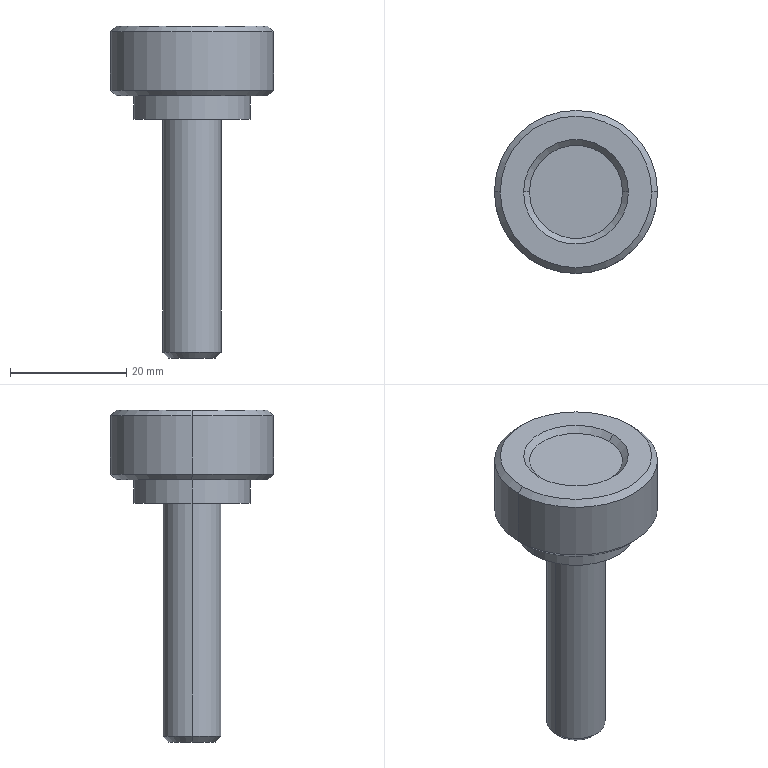Part | STEP file | Screen clamp adjusting handle | 1 solid | 23 faces | box 28 x 28 x 57 mm | volume 11437 mm3 | cone 10 | cylinder 8 | plane 5 | commonest cylinder face diameters 3.3 x2 10 x2 20 x2 28 x2
STEP:
#1=CARTESIAN_POINT('',(1.65,0.,-33.5));
#2=VERTEX_POINT('',#1);
#3=CARTESIAN_POINT('',(-1.65,0.,-33.5));
#4=VERTEX_POINT('',#3);
#5=CARTESIAN_POINT('',(0.,0.,-33.5));
#6=DIRECTION('',(0.,0.,-1.));
#7=DIRECTION('',(-1.,0.,0.));
#8=AXIS2_PLACEMENT_3D('',#5,#6,#7);
#9=CIRCLE('',#8,1.65);
#10=EDGE_CURVE('',#2,#4,#9,.T.);
#11=ORIENTED_EDGE('',*,*,#10,.F.);
#12=CARTESIAN_POINT('',(1.65,0.,-45.));
#13=VERTEX_POINT('',#12);
#14=CARTESIAN_POINT('',(1.65,0.,-45.));
#15=DIRECTION('',(0.,0.,-1.));
#16=VECTOR('',#15,1000.);
#17=LINE('',#14,#16);
#18=EDGE_CURVE('',#2,#13,#17,.T.);
#19=ORIENTED_EDGE('',*,*,#18,.T.);
#20=CARTESIAN_POINT('',(-1.65,0.,-45.));
#21=VERTEX_POINT('',#20);
#22=CARTESIAN_POINT('',(0.,0.,-45.));
#23=DIRECTION('',(0.,0.,-1.));
#24=DIRECTION('',(-1.,0.,0.));
#25=AXIS2_PLACEMENT_3D('',#22,#23,#24);
#26=CIRCLE('',#25,1.65);
#27=EDGE_CURVE('',#13,#21,#26,.T.);
#28=ORIENTED_EDGE('',*,*,#27,.T.);
#29=CARTESIAN_POINT('',(-1.65,0.,-45.));
#30=DIRECTION('',(0.,0.,-1.));
#31=VECTOR('',#30,1000.);
#32=LINE('',#29,#31);
#33=EDGE_CURVE('',#4,#21,#32,.T.);
#34=ORIENTED_EDGE('',*,*,#33,.F.);
#35=EDGE_LOOP('',(#11,#19,#28,#34));
#36=FACE_OUTER_BOUND('',#35,.T.);
#37=CARTESIAN_POINT('',(0.,0.,-45.));
#38=DIRECTION('',(0.,0.,-1.));
#39=DIRECTION('',(-1.,0.,0.));
#40=AXIS2_PLACEMENT_3D('',#37,#38,#39);
#41=CYLINDRICAL_SURFACE('',#40,1.65);
#42=ADVANCED_FACE('',(#36),#41,.F.);
#43=CARTESIAN_POINT('',(0.,0.,-32.509));
#44=VERTEX_POINT('',#43);
#45=CARTESIAN_POINT('',(-1.65,0.,-33.5));
#46=DIRECTION('',(-0.8572,0.,-0.515));
#47=VECTOR('',#46,1000.);
#48=LINE('',#45,#47);
#49=EDGE_CURVE('',#44,#4,#48,.T.);
#50=ORIENTED_EDGE('',*,*,#49,.F.);
#51=CARTESIAN_POINT('',(1.65,0.,-33.5));
#52=DIRECTION('',(0.8572,0.,-0.515));
#53=VECTOR('',#52,1000.);
#54=LINE('',#51,#53);
#55=EDGE_CURVE('',#44,#2,#54,.T.);
#56=ORIENTED_EDGE('',*,*,#55,.T.);
#57=ORIENTED_EDGE('',*,*,#10,.T.);
#58=EDGE_LOOP('',(#50,#56,#57));
#59=FACE_OUTER_BOUND('',#58,.T.);
#60=CARTESIAN_POINT('',(0.,0.,-33.5));
#61=DIRECTION('',(0.,0.,-1.));
#62=DIRECTION('',(-1.,0.,0.));
#63=AXIS2_PLACEMENT_3D('',#60,#61,#62);
#64=CONICAL_SURFACE('',#63,1.65,1.03);
#65=ADVANCED_FACE('',(#59),#64,.F.);
#66=CARTESIAN_POINT('',(-4.,0.,-45.));
#67=VERTEX_POINT('',#66);
#68=CARTESIAN_POINT('',(4.,0.,-45.));
#69=VERTEX_POINT('',#68);
#70=CARTESIAN_POINT('',(0.,0.,-45.));
#71=DIRECTION('',(0.,0.,-1.));
#72=DIRECTION('',(-1.,0.,0.));
#73=AXIS2_PLACEMENT_3D('',#70,#71,#72);
#74=CIRCLE('',#73,4.);
#75=EDGE_CURVE('',#67,#69,#74,.T.);
#76=ORIENTED_EDGE('',*,*,#75,.F.);
#77=CARTESIAN_POINT('',(-5.,0.,-44.));
#78=VERTEX_POINT('',#77);
#79=CARTESIAN_POINT('',(-4.,0.,-45.));
#80=DIRECTION('',(-0.7071,0.,0.7071));
#81=VECTOR('',#80,1000.);
#82=LINE('',#79,#81);
#83=EDGE_CURVE('',#67,#78,#82,.T.);
#84=ORIENTED_EDGE('',*,*,#83,.T.);
#85=CARTESIAN_POINT('',(5.,0.,-44.));
#86=VERTEX_POINT('',#85);
#87=CARTESIAN_POINT('',(0.,0.,-44.));
#88=DIRECTION('',(0.,0.,1.));
#89=DIRECTION('',(-1.,0.,0.));
#90=AXIS2_PLACEMENT_3D('',#87,#88,#89);
#91=CIRCLE('',#90,5.);
#92=EDGE_CURVE('',#86,#78,#91,.T.);
#93=ORIENTED_EDGE('',*,*,#92,.F.);
#94=CARTESIAN_POINT('',(4.,0.,-45.));
#95=DIRECTION('',(0.7071,0.,0.7071));
#96=VECTOR('',#95,1000.);
#97=LINE('',#94,#96);
#98=EDGE_CURVE('',#69,#86,#97,.T.);
#99=ORIENTED_EDGE('',*,*,#98,.F.);
#100=EDGE_LOOP('',(#76,#84,#93,#99));
#101=FACE_OUTER_BOUND('',#100,.T.);
#102=CARTESIAN_POINT('',(0.,0.,-45.));
#103=DIRECTION('',(0.,0.,1.));
#104=DIRECTION('',(1.,0.,0.));
#105=AXIS2_PLACEMENT_3D('',#102,#103,#104);
#106=CONICAL_SURFACE('',#105,4.,0.7854);
#107=ADVANCED_FACE('',(#101),#106,.T.);
#108=CARTESIAN_POINT('',(-13.,0.,0.));
#109=VERTEX_POINT('',#108);
#110=CARTESIAN_POINT('',(13.,0.,0.));
#111=VERTEX_POINT('',#110);
#112=CARTESIAN_POINT('',(0.,0.,0.));
#113=DIRECTION('',(0.,0.,-1.));
#114=DIRECTION('',(1.,0.,0.));
#115=AXIS2_PLACEMENT_3D('',#112,#113,#114);
#116=CIRCLE('',#115,13.);
#117=EDGE_CURVE('',#109,#111,#116,.T.);
#118=ORIENTED_EDGE('',*,*,#117,.F.);
#119=CARTESIAN_POINT('',(-14.,0.,1.));
#120=VERTEX_POINT('',#119);
#121=CARTESIAN_POINT('',(-14.,0.,1.));
#122=DIRECTION('',(-0.7071,0.,0.7071));
#123=VECTOR('',#122,1000.);
#124=LINE('',#121,#123);
#125=EDGE_CURVE('',#109,#120,#124,.T.);
#126=ORIENTED_EDGE('',*,*,#125,.T.);
#127=CARTESIAN_POINT('',(14.,0.,1.));
#128=VERTEX_POINT('',#127);
#129=CARTESIAN_POINT('',(0.,0.,1.));
#130=DIRECTION('',(0.,0.,1.));
#131=DIRECTION('',(1.,0.,0.));
#132=AXIS2_PLACEMENT_3D('',#129,#130,#131);
#133=CIRCLE('',#132,14.);
#134=EDGE_CURVE('',#128,#120,#133,.T.);
#135=ORIENTED_EDGE('',*,*,#134,.F.);
#136=CARTESIAN_POINT('',(14.,0.,1.));
#137=DIRECTION('',(0.7071,0.,0.7071));
#138=VECTOR('',#137,1000.);
#139=LINE('',#136,#138);
#140=EDGE_CURVE('',#111,#128,#139,.T.);
#141=ORIENTED_EDGE('',*,*,#140,.F.);
#142=EDGE_LOOP('',(#118,#126,#135,#141));
#143=FACE_OUTER_BOUND('',#142,.T.);
#144=CARTESIAN_POINT('',(0.,0.,1.));
#145=DIRECTION('',(0.,0.,1.));
#146=DIRECTION('',(1.,0.,0.));
#147=AXIS2_PLACEMENT_3D('',#144,#145,#146);
#148=CONICAL_SURFACE('',#147,14.,0.7854);
#149=ADVANCED_FACE('',(#143),#148,.T.);
#150=CARTESIAN_POINT('',(13.,0.,12.));
#151=VERTEX_POINT('',#150);
#152=CARTESIAN_POINT('',(-13.,0.,12.));
#153=VERTEX_POINT('',#152);
#154=CARTESIAN_POINT('',(0.,0.,12.));
#155=DIRECTION('',(0.,0.,1.));
#156=DIRECTION('',(1.,0.,0.));
#157=AXIS2_PLACEMENT_3D('',#154,#155,#156);
#158=CIRCLE('',#157,13.);
#159=EDGE_CURVE('',#151,#153,#158,.T.);
#160=ORIENTED_EDGE('',*,*,#159,.F.);
#161=CARTESIAN_POINT('',(14.,0.,11.));
#162=VERTEX_POINT('',#161);
#163=CARTESIAN_POINT('',(13.,0.,12.));
#164=DIRECTION('',(0.7071,0.,-0.7071));
#165=VECTOR('',#164,1000.);
#166=LINE('',#163,#165);
#167=EDGE_CURVE('',#151,#162,#166,.T.);
#168=ORIENTED_EDGE('',*,*,#167,.T.);
#169=CARTESIAN_POINT('',(-14.,0.,11.));
#170=VERTEX_POINT('',#169);
#171=CARTESIAN_POINT('',(0.,0.,11.));
#172=DIRECTION('',(0.,0.,-1.));
#173=DIRECTION('',(1.,0.,0.));
#174=AXIS2_PLACEMENT_3D('',#171,#172,#173);
#175=CIRCLE('',#174,14.);
#176=EDGE_CURVE('',#170,#162,#175,.T.);
#177=ORIENTED_EDGE('',*,*,#176,.F.);
#178=CARTESIAN_POINT('',(-13.,0.,12.));
#179=DIRECTION('',(-0.7071,0.,-0.7071));
#180=VECTOR('',#179,1000.);
#181=LINE('',#178,#180);
#182=EDGE_CURVE('',#153,#170,#181,.T.);
#183=ORIENTED_EDGE('',*,*,#182,.F.);
#184=EDGE_LOOP('',(#160,#168,#177,#183));
#185=FACE_OUTER_BOUND('',#184,.T.);
#186=CARTESIAN_POINT('',(0.,0.,12.));
#187=DIRECTION('',(0.,0.,-1.));
#188=DIRECTION('',(-1.,0.,0.));
#189=AXIS2_PLACEMENT_3D('',#186,#187,#188);
#190=CONICAL_SURFACE('',#189,13.,0.7854);
#191=ADVANCED_FACE('',(#185),#190,.T.);
#192=CARTESIAN_POINT('',(-8.,0.,11.));
#193=VERTEX_POINT('',#192);
#194=CARTESIAN_POINT('',(8.,0.,11.));
#195=VERTEX_POINT('',#194);
#196=CARTESIAN_POINT('',(0.,0.,11.));
#197=DIRECTION('',(0.,0.,1.));
#198=DIRECTION('',(1.,0.,0.));
#199=AXIS2_PLACEMENT_3D('',#196,#197,#198);
#200=CIRCLE('',#199,8.);
#201=EDGE_CURVE('',#193,#195,#200,.T.);
#202=ORIENTED_EDGE('',*,*,#201,.F.);
#203=CARTESIAN_POINT('',(-9.,0.,12.));
#204=VERTEX_POINT('',#203);
#205=CARTESIAN_POINT('',(-8.,0.,11.));
#206=DIRECTION('',(-0.7071,0.,0.7071));
#207=VECTOR('',#206,1000.);
#208=LINE('',#205,#207);
#209=EDGE_CURVE('',#193,#204,#208,.T.);
#210=ORIENTED_EDGE('',*,*,#209,.T.);
#211=CARTESIAN_POINT('',(9.,0.,12.));
#212=VERTEX_POINT('',#211);
#213=CARTESIAN_POINT('',(0.,0.,12.));
#214=DIRECTION('',(0.,0.,-1.));
#215=DIRECTION('',(1.,0.,0.));
#216=AXIS2_PLACEMENT_3D('',#213,#214,#215);
#217=CIRCLE('',#216,9.);
#218=EDGE_CURVE('',#212,#204,#217,.T.);
#219=ORIENTED_EDGE('',*,*,#218,.F.);
#220=CARTESIAN_POINT('',(8.,0.,11.));
#221=DIRECTION('',(0.7071,0.,0.7071));
#222=VECTOR('',#221,1000.);
#223=LINE('',#220,#222);
#224=EDGE_CURVE('',#195,#212,#223,.T.);
#225=ORIENTED_EDGE('',*,*,#224,.F.);
#226=EDGE_LOOP('',(#202,#210,#219,#225));
#227=FACE_OUTER_BOUND('',#226,.T.);
#228=CARTESIAN_POINT('',(0.,0.,11.));
#229=DIRECTION('',(0.,0.,1.));
#230=DIRECTION('',(1.,0.,0.));
#231=AXIS2_PLACEMENT_3D('',#228,#229,#230);
#232=CONICAL_SURFACE('',#231,8.,0.7854);
#233=ADVANCED_FACE('',(#227),#232,.F.);
#234=ORIENTED_EDGE('',*,*,#92,.T.);
#235=CARTESIAN_POINT('',(-5.,0.,-4.));
#236=VERTEX_POINT('',#235);
#237=CARTESIAN_POINT('',(-5.,0.,-45.));
#238=DIRECTION('',(0.,0.,1.));
#239=VECTOR('',#238,1000.);
#240=LINE('',#237,#239);
#241=EDGE_CURVE('',#78,#236,#240,.T.);
#242=ORIENTED_EDGE('',*,*,#241,.T.);
#243=CARTESIAN_POINT('',(5.,0.,-4.));
#244=VERTEX_POINT('',#243);
#245=CARTESIAN_POINT('',(0.,0.,-4.));
#246=DIRECTION('',(0.,0.,-1.));
#247=DIRECTION('',(-1.,0.,0.));
#248=AXIS2_PLACEMENT_3D('',#245,#246,#247);
#249=CIRCLE('',#248,5.);
#250=EDGE_CURVE('',#236,#244,#249,.T.);
#251=ORIENTED_EDGE('',*,*,#250,.T.);
#252=CARTESIAN_POINT('',(5.,0.,-45.));
#253=DIRECTION('',(0.,0.,1.));
#254=VECTOR('',#253,1000.);
#255=LINE('',#252,#254);
#256=EDGE_CURVE('',#86,#244,#255,.T.);
#257=ORIENTED_EDGE('',*,*,#256,.F.);
#258=EDGE_LOOP('',(#234,#242,#251,#257));
#259=FACE_OUTER_BOUND('',#258,.T.);
#260=CARTESIAN_POINT('',(0.,0.,-45.));
#261=DIRECTION('',(0.,0.,1.));
#262=DIRECTION('',(1.,0.,0.));
#263=AXIS2_PLACEMENT_3D('',#260,#261,#262);
#264=CYLINDRICAL_SURFACE('',#263,5.);
#265=ADVANCED_FACE('',(#259),#264,.T.);
#266=CARTESIAN_POINT('',(-10.,0.,-4.));
#267=VERTEX_POINT('',#266);
#268=CARTESIAN_POINT('',(10.,0.,-4.));
#269=VERTEX_POINT('',#268);
#270=CARTESIAN_POINT('',(0.,0.,-4.));
#271=DIRECTION('',(0.,0.,-1.));
#272=DIRECTION('',(-1.,0.,0.));
#273=AXIS2_PLACEMENT_3D('',#270,#271,#272);
#274=CIRCLE('',#273,10.);
#275=EDGE_CURVE('',#267,#269,#274,.T.);
#276=ORIENTED_EDGE('',*,*,#275,.F.);
#277=CARTESIAN_POINT('',(-10.,0.,0.));
#278=VERTEX_POINT('',#277);
#279=CARTESIAN_POINT('',(-10.,0.,-4.));
#280=DIRECTION('',(0.,0.,1.));
#281=VECTOR('',#280,1000.);
#282=LINE('',#279,#281);
#283=EDGE_CURVE('',#267,#278,#282,.T.);
#284=ORIENTED_EDGE('',*,*,#283,.T.);
#285=CARTESIAN_POINT('',(10.,0.,0.));
#286=VERTEX_POINT('',#285);
#287=CARTESIAN_POINT('',(0.,0.,0.));
#288=DIRECTION('',(0.,0.,-1.));
#289=DIRECTION('',(1.,0.,0.));
#290=AXIS2_PLACEMENT_3D('',#287,#288,#289);
#291=CIRCLE('',#290,10.);
#292=EDGE_CURVE('',#278,#286,#291,.T.);
#293=ORIENTED_EDGE('',*,*,#292,.T.);
#294=CARTESIAN_POINT('',(10.,0.,-4.));
#295=DIRECTION('',(0.,0.,1.));
#296=VECTOR('',#295,1000.);
#297=LINE('',#294,#296);
#298=EDGE_CURVE('',#269,#286,#297,.T.);
#299=ORIENTED_EDGE('',*,*,#298,.F.);
#300=EDGE_LOOP('',(#276,#284,#293,#299));
#301=FACE_OUTER_BOUND('',#300,.T.);
#302=CARTESIAN_POINT('',(0.,0.,-4.));
#303=DIRECTION('',(0.,0.,1.));
#304=DIRECTION('',(1.,0.,0.));
#305=AXIS2_PLACEMENT_3D('',#302,#303,#304);
#306=CYLINDRICAL_SURFACE('',#305,10.);
#307=ADVANCED_FACE('',(#301),#306,.T.);
#308=ORIENTED_EDGE('',*,*,#176,.T.);
#309=CARTESIAN_POINT('',(14.,0.,12.));
#310=DIRECTION('',(0.,0.,-1.));
#311=VECTOR('',#310,1000.);
#312=LINE('',#309,#311);
#313=EDGE_CURVE('',#162,#128,#312,.T.);
#314=ORIENTED_EDGE('',*,*,#313,.T.);
#315=ORIENTED_EDGE('',*,*,#134,.T.);
#316=CARTESIAN_POINT('',(-14.,0.,12.));
#317=DIRECTION('',(0.,0.,-1.));
#318=VECTOR('',#317,1000.);
#319=LINE('',#316,#318);
#320=EDGE_CURVE('',#170,#120,#319,.T.);
#321=ORIENTED_EDGE('',*,*,#320,.F.);
#322=EDGE_LOOP('',(#308,#314,#315,#321));
#323=FACE_OUTER_BOUND('',#322,.T.);
#324=CARTESIAN_POINT('',(0.,0.,12.));
#325=DIRECTION('',(0.,0.,-1.));
#326=DIRECTION('',(-1.,0.,0.));
#327=AXIS2_PLACEMENT_3D('',#324,#325,#326);
#328=CYLINDRICAL_SURFACE('',#327,14.);
#329=ADVANCED_FACE('',(#323),#328,.T.);
#330=CARTESIAN_POINT('',(0.,0.,0.));
#331=DIRECTION('',(0.,0.,-1.));
#332=DIRECTION('',(1.,0.,0.));
#333=AXIS2_PLACEMENT_3D('',#330,#331,#332);
#334=CIRCLE('',#333,13.);
#335=EDGE_CURVE('',#111,#109,#334,.T.);
#336=ORIENTED_EDGE('',*,*,#335,.T.);
#337=ORIENTED_EDGE('',*,*,#117,.T.);
#338=EDGE_LOOP('',(#336,#337));
#339=FACE_OUTER_BOUND('',#338,.T.);
#340=CARTESIAN_POINT('',(0.,0.,0.));
#341=DIRECTION('',(0.,0.,-1.));
#342=DIRECTION('',(1.,0.,0.));
#343=AXIS2_PLACEMENT_3D('',#340,#341,#342);
#344=CIRCLE('',#343,10.);
#345=EDGE_CURVE('',#286,#278,#344,.T.);
#346=ORIENTED_EDGE('',*,*,#345,.F.);
#347=ORIENTED_EDGE('',*,*,#292,.F.);
#348=EDGE_LOOP('',(#346,#347));
#349=FACE_BOUND('',#348,.T.);
#350=CARTESIAN_POINT('',(0.,0.,0.));
#351=DIRECTION('',(0.,0.,1.));
#352=DIRECTION('',(1.,0.,0.));
#353=AXIS2_PLACEMENT_3D('',#350,#351,#352);
#354=PLANE('',#353);
#355=ADVANCED_FACE('',(#339,#349),#354,.F.);
#356=ORIENTED_EDGE('',*,*,#313,.F.);
#357=CARTESIAN_POINT('',(0.,0.,11.));
#358=DIRECTION('',(0.,0.,-1.));
#359=DIRECTION('',(1.,0.,0.));
#360=AXIS2_PLACEMENT_3D('',#357,#358,#359);
#361=CIRCLE('',#360,14.);
#362=EDGE_CURVE('',#162,#170,#361,.T.);
#363=ORIENTED_EDGE('',*,*,#362,.T.);
#364=ORIENTED_EDGE('',*,*,#320,.T.);
#365=CARTESIAN_POINT('',(0.,0.,1.));
#366=DIRECTION('',(0.,0.,1.));
#367=DIRECTION('',(1.,0.,0.));
#368=AXIS2_PLACEMENT_3D('',#365,#366,#367);
#369=CIRCLE('',#368,14.);
#370=EDGE_CURVE('',#120,#128,#369,.T.);
#371=ORIENTED_EDGE('',*,*,#370,.T.);
#372=EDGE_LOOP('',(#356,#363,#364,#371));
#373=FACE_OUTER_BOUND('',#372,.T.);
#374=CARTESIAN_POINT('',(0.,0.,12.));
#375=DIRECTION('',(0.,0.,-1.));
#376=DIRECTION('',(-1.,0.,0.));
#377=AXIS2_PLACEMENT_3D('',#374,#375,#376);
#378=CYLINDRICAL_SURFACE('',#377,14.);
#379=ADVANCED_FACE('',(#373),#378,.T.);
#380=ORIENTED_EDGE('',*,*,#218,.T.);
#381=CARTESIAN_POINT('',(0.,0.,12.));
#382=DIRECTION('',(0.,0.,-1.));
#383=DIRECTION('',(1.,0.,0.));
#384=AXIS2_PLACEMENT_3D('',#381,#382,#383);
#385=CIRCLE('',#384,9.);
#386=EDGE_CURVE('',#204,#212,#385,.T.);
#387=ORIENTED_EDGE('',*,*,#386,.T.);
#388=EDGE_LOOP('',(#380,#387));
#389=FACE_BOUND('',#388,.T.);
#390=CARTESIAN_POINT('',(0.,0.,12.));
#391=DIRECTION('',(0.,0.,1.));
#392=DIRECTION('',(1.,0.,0.));
#393=AXIS2_PLACEMENT_3D('',#390,#391,#392);
#394=CIRCLE('',#393,13.);
#395=EDGE_CURVE('',#153,#151,#394,.T.);
#396=ORIENTED_EDGE('',*,*,#395,.T.);
#397=ORIENTED_EDGE('',*,*,#159,.T.);
#398=EDGE_LOOP('',(#396,#397));
#399=FACE_OUTER_BOUND('',#398,.T.);
#400=CARTESIAN_POINT('',(0.,0.,12.));
#401=DIRECTION('',(0.,0.,1.));
#402=DIRECTION('',(1.,0.,0.));
#403=AXIS2_PLACEMENT_3D('',#400,#401,#402);
#404=PLANE('',#403);
#405=ADVANCED_FACE('',(#389,#399),#404,.T.);
#406=CARTESIAN_POINT('',(0.,0.,-4.));
#407=DIRECTION('',(0.,0.,-1.));
#408=DIRECTION('',(-1.,0.,0.));
#409=AXIS2_PLACEMENT_3D('',#406,#407,#408);
#410=CIRCLE('',#409,10.);
#411=EDGE_CURVE('',#269,#267,#410,.T.);
#412=ORIENTED_EDGE('',*,*,#411,.T.);
#413=ORIENTED_EDGE('',*,*,#275,.T.);
#414=EDGE_LOOP('',(#412,#413));
#415=FACE_OUTER_BOUND('',#414,.T.);
#416=CARTESIAN_POINT('',(0.,0.,-4.));
#417=DIRECTION('',(0.,0.,-1.));
#418=DIRECTION('',(-1.,0.,0.));
#419=AXIS2_PLACEMENT_3D('',#416,#417,#418);
#420=CIRCLE('',#419,5.);
#421=EDGE_CURVE('',#244,#236,#420,.T.);
#422=ORIENTED_EDGE('',*,*,#421,.F.);
#423=ORIENTED_EDGE('',*,*,#250,.F.);
#424=EDGE_LOOP('',(#422,#423));
#425=FACE_BOUND('',#424,.T.);
#426=CARTESIAN_POINT('',(0.,0.,-4.));
#427=DIRECTION('',(0.,0.,-1.));
#428=DIRECTION('',(-1.,0.,0.));
#429=AXIS2_PLACEMENT_3D('',#426,#427,#428);
#430=PLANE('',#429);
#431=ADVANCED_FACE('',(#415,#425),#430,.T.);
#432=ORIENTED_EDGE('',*,*,#283,.F.);
#433=ORIENTED_EDGE('',*,*,#411,.F.);
#434=ORIENTED_EDGE('',*,*,#298,.T.);
#435=ORIENTED_EDGE('',*,*,#345,.T.);
#436=EDGE_LOOP('',(#432,#433,#434,#435));
#437=FACE_OUTER_BOUND('',#436,.T.);
#438=CARTESIAN_POINT('',(0.,0.,-4.));
#439=DIRECTION('',(0.,0.,1.));
#440=DIRECTION('',(1.,0.,0.));
#441=AXIS2_PLACEMENT_3D('',#438,#439,#440);
#442=CYLINDRICAL_SURFACE('',#441,10.);
#443=ADVANCED_FACE('',(#437),#442,.T.);
#444=CARTESIAN_POINT('',(0.,0.,-45.));
#445=DIRECTION('',(0.,0.,-1.));
#446=DIRECTION('',(-1.,0.,0.));
#447=AXIS2_PLACEMENT_3D('',#444,#445,#446);
#448=CIRCLE('',#447,1.65);
#449=EDGE_CURVE('',#21,#13,#448,.T.);
#450=ORIENTED_EDGE('',*,*,#449,.F.);
#451=ORIENTED_EDGE('',*,*,#27,.F.);
#452=EDGE_LOOP('',(#450,#451));
#453=FACE_BOUND('',#452,.T.);
#454=CARTESIAN_POINT('',(0.,0.,-45.));
#455=DIRECTION('',(0.,0.,-1.));
#456=DIRECTION('',(-1.,0.,0.));
#457=AXIS2_PLACEMENT_3D('',#454,#455,#456);
#458=CIRCLE('',#457,4.);
#459=EDGE_CURVE('',#69,#67,#458,.T.);
#460=ORIENTED_EDGE('',*,*,#459,.T.);
#461=ORIENTED_EDGE('',*,*,#75,.T.);
#462=EDGE_LOOP('',(#460,#461));
#463=FACE_OUTER_BOUND('',#462,.T.);
#464=CARTESIAN_POINT('',(0.,0.,-45.));
#465=DIRECTION('',(0.,0.,-1.));
#466=DIRECTION('',(-1.,0.,0.));
#467=AXIS2_PLACEMENT_3D('',#464,#465,#466);
#468=PLANE('',#467);
#469=ADVANCED_FACE('',(#453,#463),#468,.T.);
#470=ORIENTED_EDGE('',*,*,#241,.F.);
#471=CARTESIAN_POINT('',(0.,0.,-44.));
#472=DIRECTION('',(0.,0.,1.));
#473=DIRECTION('',(-1.,0.,0.));
#474=AXIS2_PLACEMENT_3D('',#471,#472,#473);
#475=CIRCLE('',#474,5.);
#476=EDGE_CURVE('',#78,#86,#475,.T.);
#477=ORIENTED_EDGE('',*,*,#476,.T.);
#478=ORIENTED_EDGE('',*,*,#256,.T.);
#479=ORIENTED_EDGE('',*,*,#421,.T.);
#480=EDGE_LOOP('',(#470,#477,#478,#479));
#481=FACE_OUTER_BOUND('',#480,.T.);
#482=CARTESIAN_POINT('',(0.,0.,-45.));
#483=DIRECTION('',(0.,0.,1.));
#484=DIRECTION('',(1.,0.,0.));
#485=AXIS2_PLACEMENT_3D('',#482,#483,#484);
#486=CYLINDRICAL_SURFACE('',#485,5.);
#487=ADVANCED_FACE('',(#481),#486,.T.);
#488=CARTESIAN_POINT('',(0.,0.,11.));
#489=DIRECTION('',(0.,0.,1.));
#490=DIRECTION('',(1.,0.,0.));
#491=AXIS2_PLACEMENT_3D('',#488,#489,#490);
#492=CIRCLE('',#491,8.);
#493=EDGE_CURVE('',#195,#193,#492,.T.);
#494=ORIENTED_EDGE('',*,*,#493,.T.);
#495=ORIENTED_EDGE('',*,*,#201,.T.);
#496=EDGE_LOOP('',(#494,#495));
#497=FACE_OUTER_BOUND('',#496,.T.);
#498=CARTESIAN_POINT('',(0.,0.,11.));
#499=DIRECTION('',(0.,0.,1.));
#500=DIRECTION('',(1.,0.,0.));
#501=AXIS2_PLACEMENT_3D('',#498,#499,#500);
#502=PLANE('',#501);
#503=ADVANCED_FACE('',(#497),#502,.T.);
#504=ORIENTED_EDGE('',*,*,#209,.F.);
#505=ORIENTED_EDGE('',*,*,#493,.F.);
#506=ORIENTED_EDGE('',*,*,#224,.T.);
#507=ORIENTED_EDGE('',*,*,#386,.F.);
#508=EDGE_LOOP('',(#504,#505,#506,#507));
#509=FACE_OUTER_BOUND('',#508,.T.);
#510=CARTESIAN_POINT('',(0.,0.,11.));
#511=DIRECTION('',(0.,0.,1.));
#512=DIRECTION('',(1.,0.,0.));
#513=AXIS2_PLACEMENT_3D('',#510,#511,#512);
#514=CONICAL_SURFACE('',#513,8.,0.7854);
#515=ADVANCED_FACE('',(#509),#514,.F.);
#516=ORIENTED_EDGE('',*,*,#167,.F.);
#517=ORIENTED_EDGE('',*,*,#395,.F.);
#518=ORIENTED_EDGE('',*,*,#182,.T.);
#519=ORIENTED_EDGE('',*,*,#362,.F.);
#520=EDGE_LOOP('',(#516,#517,#518,#519));
#521=FACE_OUTER_BOUND('',#520,.T.);
#522=CARTESIAN_POINT('',(0.,0.,12.));
#523=DIRECTION('',(0.,0.,-1.));
#524=DIRECTION('',(-1.,0.,0.));
#525=AXIS2_PLACEMENT_3D('',#522,#523,#524);
#526=CONICAL_SURFACE('',#525,13.,0.7854);
#527=ADVANCED_FACE('',(#521),#526,.T.);
#528=ORIENTED_EDGE('',*,*,#125,.F.);
#529=ORIENTED_EDGE('',*,*,#335,.F.);
#530=ORIENTED_EDGE('',*,*,#140,.T.);
#531=ORIENTED_EDGE('',*,*,#370,.F.);
#532=EDGE_LOOP('',(#528,#529,#530,#531));
#533=FACE_OUTER_BOUND('',#532,.T.);
#534=CARTESIAN_POINT('',(0.,0.,1.));
#535=DIRECTION('',(0.,0.,1.));
#536=DIRECTION('',(1.,0.,0.));
#537=AXIS2_PLACEMENT_3D('',#534,#535,#536);
#538=CONICAL_SURFACE('',#537,14.,0.7854);
#539=ADVANCED_FACE('',(#533),#538,.T.);
#540=ORIENTED_EDGE('',*,*,#83,.F.);
#541=ORIENTED_EDGE('',*,*,#459,.F.);
#542=ORIENTED_EDGE('',*,*,#98,.T.);
#543=ORIENTED_EDGE('',*,*,#476,.F.);
#544=EDGE_LOOP('',(#540,#541,#542,#543));
#545=FACE_OUTER_BOUND('',#544,.T.);
#546=CARTESIAN_POINT('',(0.,0.,-45.));
#547=DIRECTION('',(0.,0.,1.));
#548=DIRECTION('',(1.,0.,0.));
#549=AXIS2_PLACEMENT_3D('',#546,#547,#548);
#550=CONICAL_SURFACE('',#549,4.,0.7854);
#551=ADVANCED_FACE('',(#545),#550,.T.);
#552=ORIENTED_EDGE('',*,*,#55,.F.);
#553=ORIENTED_EDGE('',*,*,#49,.T.);
#554=CARTESIAN_POINT('',(0.,0.,-33.5));
#555=DIRECTION('',(0.,0.,-1.));
#556=DIRECTION('',(-1.,0.,0.));
#557=AXIS2_PLACEMENT_3D('',#554,#555,#556);
#558=CIRCLE('',#557,1.65);
#559=EDGE_CURVE('',#4,#2,#558,.T.);
#560=ORIENTED_EDGE('',*,*,#559,.T.);
#561=EDGE_LOOP('',(#552,#553,#560));
#562=FACE_OUTER_BOUND('',#561,.T.);
#563=CARTESIAN_POINT('',(0.,0.,-33.5));
#564=DIRECTION('',(0.,0.,-1.));
#565=DIRECTION('',(-1.,0.,0.));
#566=AXIS2_PLACEMENT_3D('',#563,#564,#565);
#567=CONICAL_SURFACE('',#566,1.65,1.03);
#568=ADVANCED_FACE('',(#562),#567,.F.);
#569=ORIENTED_EDGE('',*,*,#18,.F.);
#570=ORIENTED_EDGE('',*,*,#559,.F.);
#571=ORIENTED_EDGE('',*,*,#33,.T.);
#572=ORIENTED_EDGE('',*,*,#449,.T.);
#573=EDGE_LOOP('',(#569,#570,#571,#572));
#574=FACE_OUTER_BOUND('',#573,.T.);
#575=CARTESIAN_POINT('',(0.,0.,-45.));
#576=DIRECTION('',(0.,0.,-1.));
#577=DIRECTION('',(-1.,0.,0.));
#578=AXIS2_PLACEMENT_3D('',#575,#576,#577);
#579=CYLINDRICAL_SURFACE('',#578,1.65);
#580=ADVANCED_FACE('',(#574),#579,.F.);
#581=CLOSED_SHELL('',(#42,#65,#107,#149,#191,#233,#265,#307,#329,#355,#379,#405,#431,#443,#469,#487,#503,#515,#527,#539,#551,#568,#580));
#582=MANIFOLD_SOLID_BREP('',#581);
#583=CARTESIAN_POINT('',(0.,0.,0.));
#584=DIRECTION('',(0.,0.,1.));
#585=DIRECTION('',(1.,0.,0.));
#586=AXIS2_PLACEMENT_3D('',#583,#584,#585);
#587=(LENGTH_UNIT()NAMED_UNIT(*)SI_UNIT(.MILLI.,.METRE.));
#588=UNCERTAINTY_MEASURE_WITH_UNIT(LENGTH_MEASURE(0.00001),#587,'','');
#589=(NAMED_UNIT(*)PLANE_ANGLE_UNIT()SI_UNIT($,.RADIAN.));
#590=(NAMED_UNIT(*)SI_UNIT($,.STERADIAN.)SOLID_ANGLE_UNIT());
#591=(GEOMETRIC_REPRESENTATION_CONTEXT(3)GLOBAL_UNCERTAINTY_ASSIGNED_CONTEXT((#588))GLOBAL_UNIT_ASSIGNED_CONTEXT((#587,#589,#590))REPRESENTATION_CONTEXT('',''));
#592=ADVANCED_BREP_SHAPE_REPRESENTATION('',(#582,#586),#591);